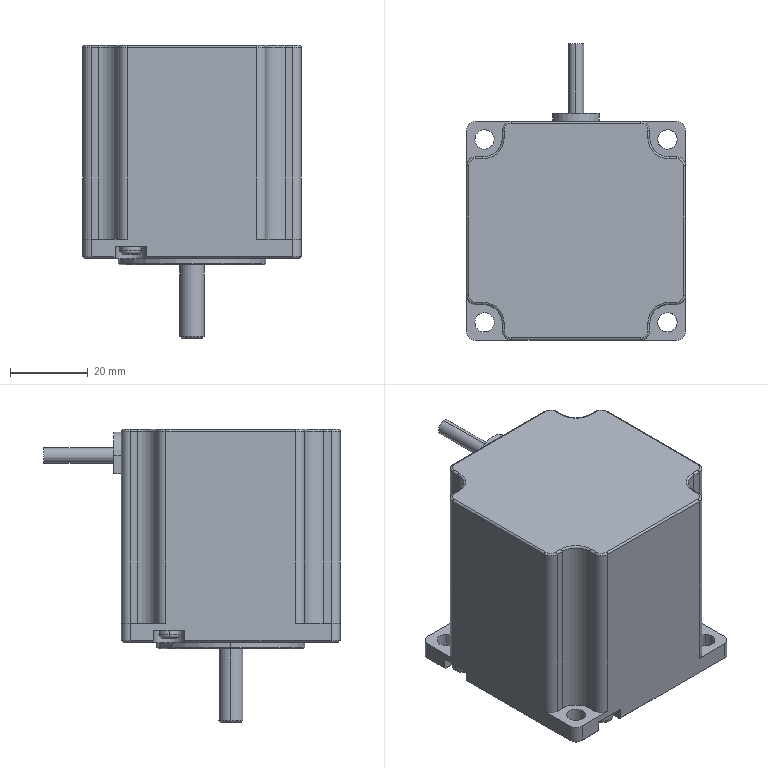Part | STEP file | HSTM57-1.8-S-56 | 1 solid | 196 faces | box 56.438 x 76.419 x 75.6 mm | volume 160609 mm3 | plane 106 | cylinder 62 | torus 20 | cone 8 | commonest cylinder face diameters 5 x14 1 x12 4.6 x12 5.5 x8 8 x5 10 x4